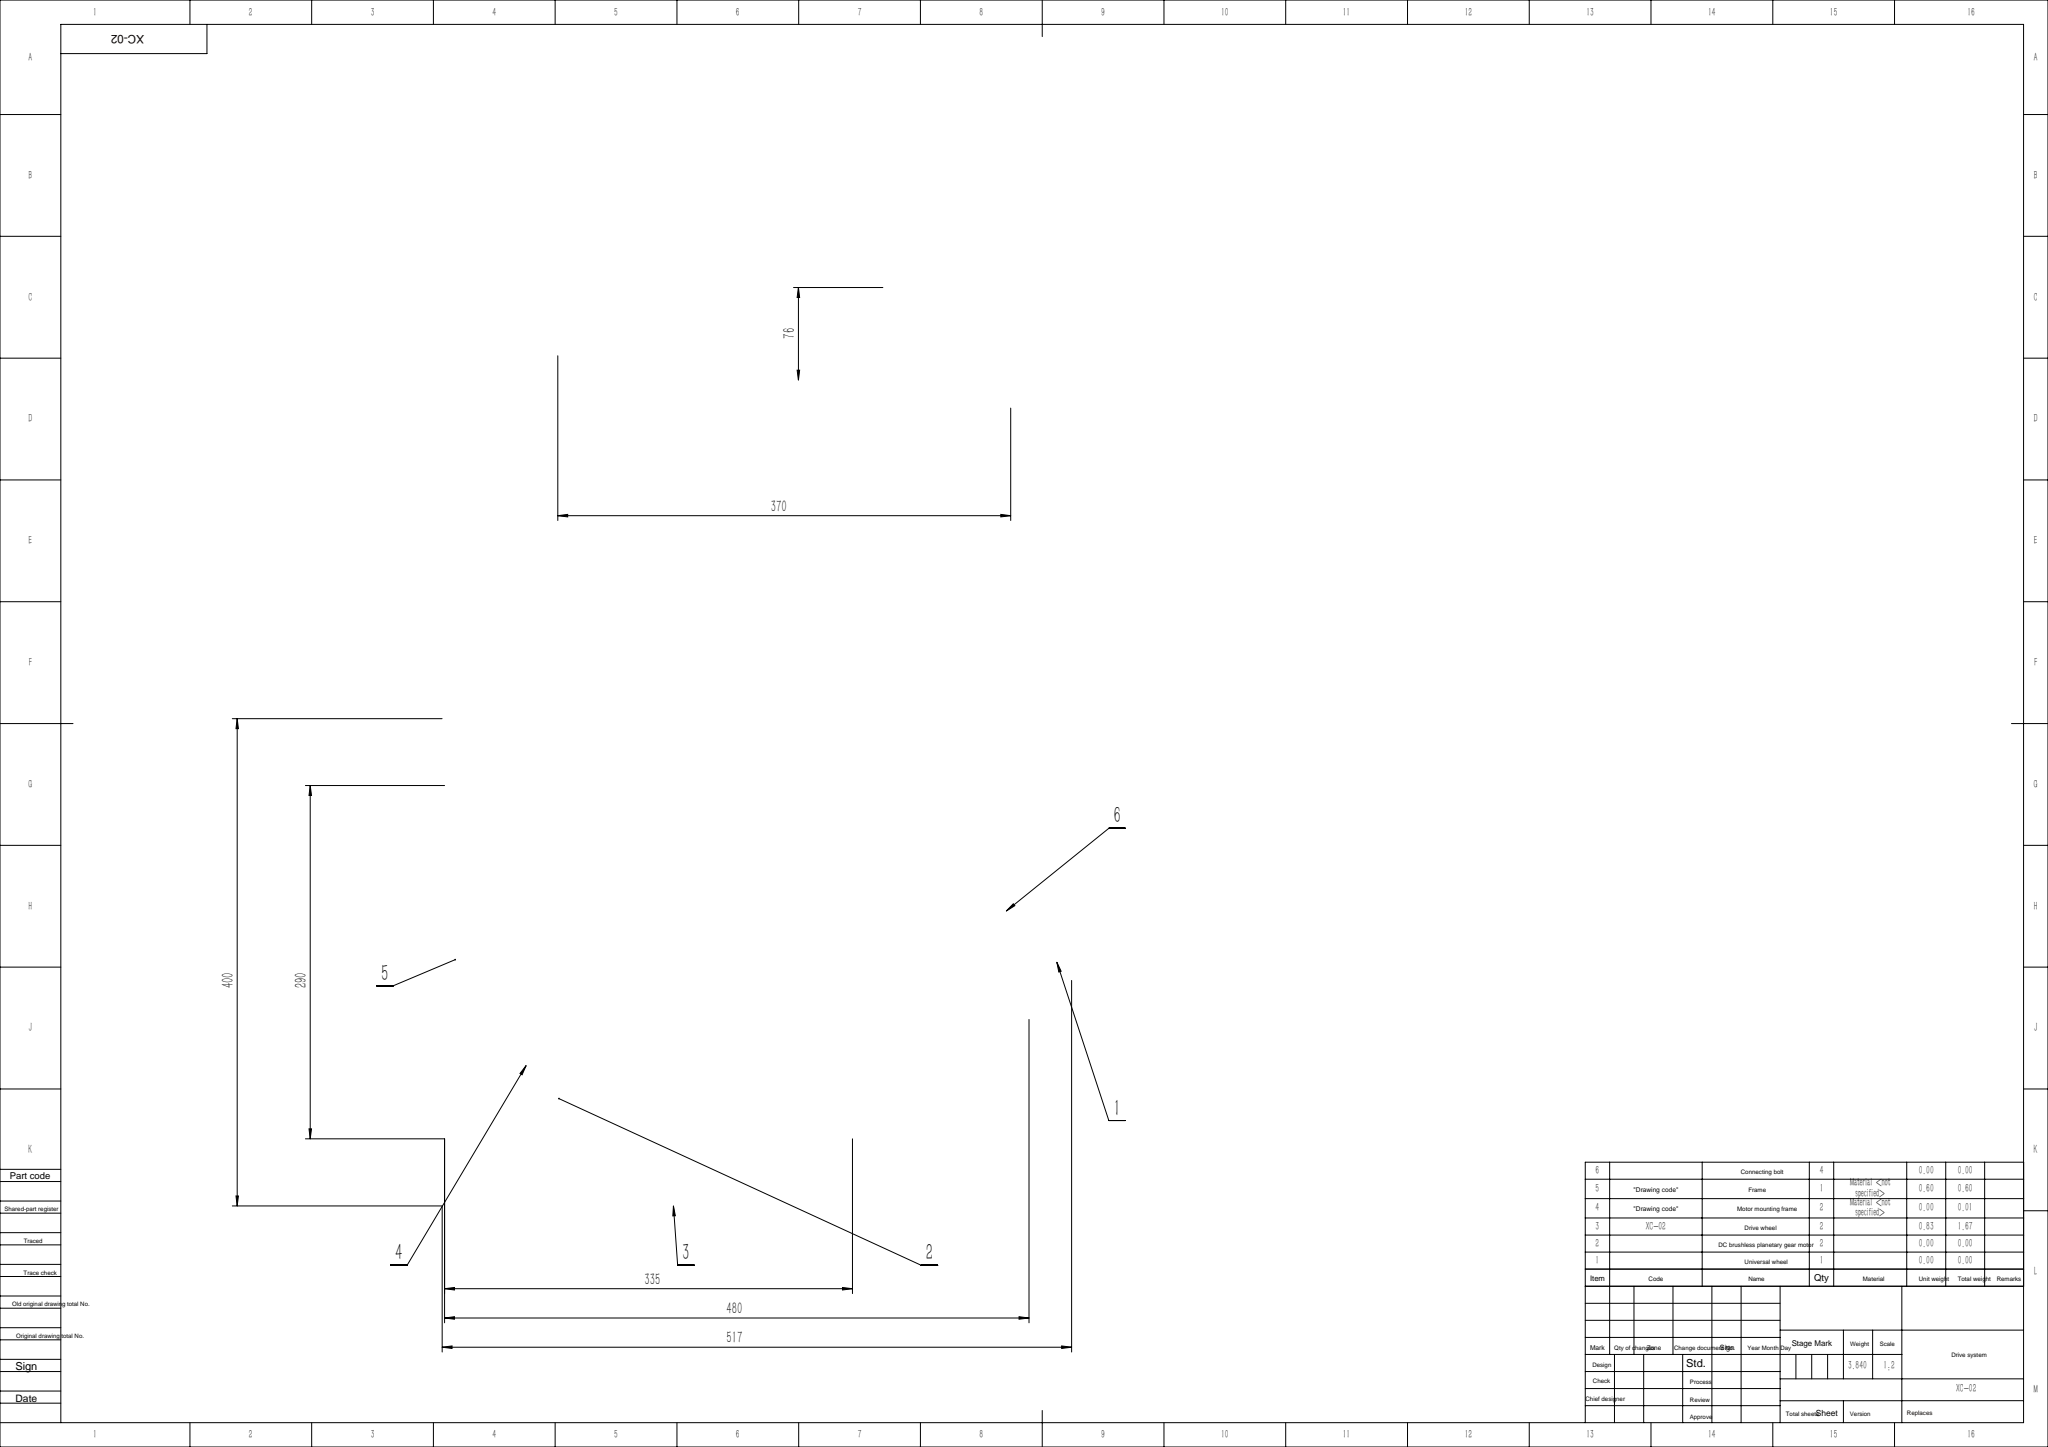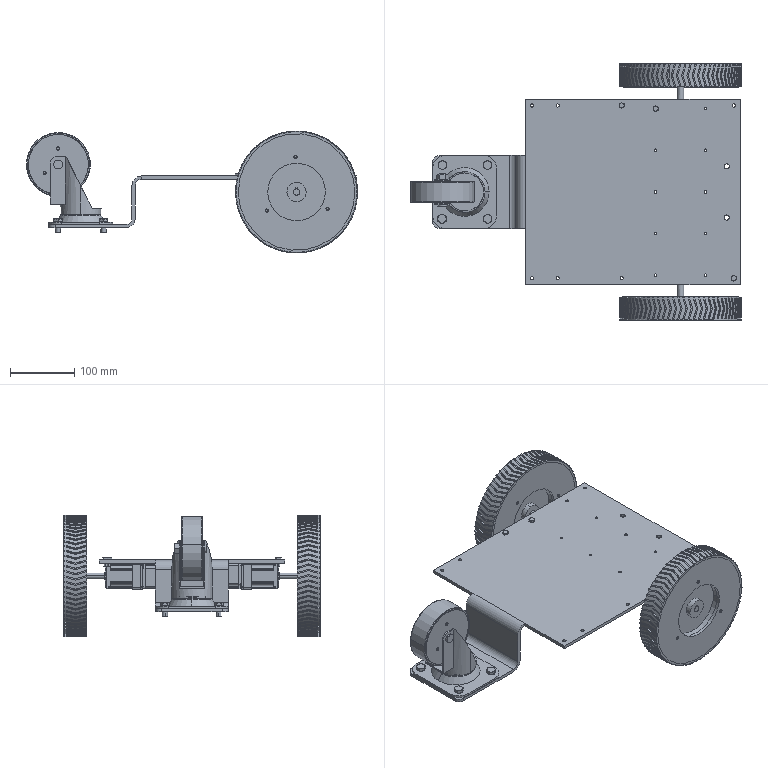Part | SolidWorks | features CompositeCurve 2, LocalLPattern 1 | 53 solids | 2374 faces | box 517.127 x 400 x 190.253 mm | volume 2987569 mm3 | plane 1250 | cylinder 736 | torus 132 | cone 118 | spline 70 | sphere 68 | commonest cylinder face diameters 188 x146 5 x100 4 x52 8 x44 0.6 x34 2 x26